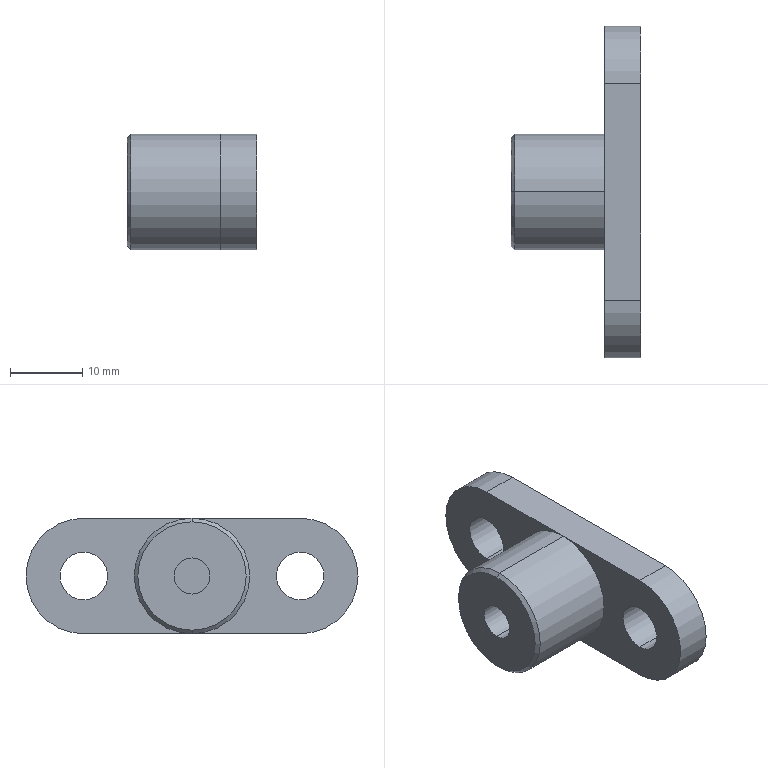Part | STEP file | HJDX-008 | 1 solid | 19 faces | box 18 x 46 x 16 mm | volume 5416 mm3 | cylinder 10 | plane 7 | cone 2 | commonest cylinder face diameters 6.6 x4 16 x4 5 x2
STEP:
#1=CARTESIAN_POINT('',(18.,-15.,-3.3));
#2=VERTEX_POINT('',#1);
#3=CARTESIAN_POINT('',(18.,-15.,3.3));
#4=VERTEX_POINT('',#3);
#5=CARTESIAN_POINT('',(18.,-15.,0.));
#6=DIRECTION('',(-1.,0.,0.));
#7=DIRECTION('',(0.,0.,1.));
#8=AXIS2_PLACEMENT_3D('',#5,#6,#7);
#9=CIRCLE('',#8,3.3);
#10=EDGE_CURVE('',#2,#4,#9,.T.);
#11=ORIENTED_EDGE('',*,*,#10,.F.);
#12=CARTESIAN_POINT('',(13.,-15.,-3.3));
#13=VERTEX_POINT('',#12);
#14=CARTESIAN_POINT('',(13.,-15.,-3.3));
#15=DIRECTION('',(-1.,0.,0.));
#16=VECTOR('',#15,1000.);
#17=LINE('',#14,#16);
#18=EDGE_CURVE('',#2,#13,#17,.T.);
#19=ORIENTED_EDGE('',*,*,#18,.T.);
#20=CARTESIAN_POINT('',(13.,-15.,3.3));
#21=VERTEX_POINT('',#20);
#22=CARTESIAN_POINT('',(13.,-15.,0.));
#23=DIRECTION('',(1.,0.,0.));
#24=DIRECTION('',(0.,0.,1.));
#25=AXIS2_PLACEMENT_3D('',#22,#23,#24);
#26=CIRCLE('',#25,3.3);
#27=EDGE_CURVE('',#21,#13,#26,.T.);
#28=ORIENTED_EDGE('',*,*,#27,.F.);
#29=CARTESIAN_POINT('',(13.,-15.,3.3));
#30=DIRECTION('',(-1.,0.,0.));
#31=VECTOR('',#30,1000.);
#32=LINE('',#29,#31);
#33=EDGE_CURVE('',#4,#21,#32,.T.);
#34=ORIENTED_EDGE('',*,*,#33,.F.);
#35=EDGE_LOOP('',(#11,#19,#28,#34));
#36=FACE_OUTER_BOUND('',#35,.T.);
#37=CARTESIAN_POINT('',(13.,-15.,0.));
#38=DIRECTION('',(-1.,0.,0.));
#39=DIRECTION('',(0.,0.,1.));
#40=AXIS2_PLACEMENT_3D('',#37,#38,#39);
#41=CYLINDRICAL_SURFACE('',#40,3.3);
#42=ADVANCED_FACE('',(#36),#41,.F.);
#43=CARTESIAN_POINT('',(18.,15.,-3.3));
#44=VERTEX_POINT('',#43);
#45=CARTESIAN_POINT('',(18.,15.,3.3));
#46=VERTEX_POINT('',#45);
#47=CARTESIAN_POINT('',(18.,15.,0.));
#48=DIRECTION('',(-1.,0.,0.));
#49=DIRECTION('',(0.,0.,1.));
#50=AXIS2_PLACEMENT_3D('',#47,#48,#49);
#51=CIRCLE('',#50,3.3);
#52=EDGE_CURVE('',#44,#46,#51,.T.);
#53=ORIENTED_EDGE('',*,*,#52,.F.);
#54=CARTESIAN_POINT('',(13.,15.,-3.3));
#55=VERTEX_POINT('',#54);
#56=CARTESIAN_POINT('',(13.,15.,-3.3));
#57=DIRECTION('',(-1.,0.,0.));
#58=VECTOR('',#57,1000.);
#59=LINE('',#56,#58);
#60=EDGE_CURVE('',#44,#55,#59,.T.);
#61=ORIENTED_EDGE('',*,*,#60,.T.);
#62=CARTESIAN_POINT('',(13.,15.,3.3));
#63=VERTEX_POINT('',#62);
#64=CARTESIAN_POINT('',(13.,15.,0.));
#65=DIRECTION('',(1.,0.,0.));
#66=DIRECTION('',(0.,0.,1.));
#67=AXIS2_PLACEMENT_3D('',#64,#65,#66);
#68=CIRCLE('',#67,3.3);
#69=EDGE_CURVE('',#63,#55,#68,.T.);
#70=ORIENTED_EDGE('',*,*,#69,.F.);
#71=CARTESIAN_POINT('',(13.,15.,3.3));
#72=DIRECTION('',(-1.,0.,0.));
#73=VECTOR('',#72,1000.);
#74=LINE('',#71,#73);
#75=EDGE_CURVE('',#46,#63,#74,.T.);
#76=ORIENTED_EDGE('',*,*,#75,.F.);
#77=EDGE_LOOP('',(#53,#61,#70,#76));
#78=FACE_OUTER_BOUND('',#77,.T.);
#79=CARTESIAN_POINT('',(13.,15.,0.));
#80=DIRECTION('',(-1.,0.,0.));
#81=DIRECTION('',(0.,0.,1.));
#82=AXIS2_PLACEMENT_3D('',#79,#80,#81);
#83=CYLINDRICAL_SURFACE('',#82,3.3);
#84=ADVANCED_FACE('',(#78),#83,.F.);
#85=CARTESIAN_POINT('',(13.,0.,8.));
#86=VERTEX_POINT('',#85);
#87=CARTESIAN_POINT('',(13.,0.,-8.));
#88=VERTEX_POINT('',#87);
#89=CARTESIAN_POINT('',(13.,0.,0.));
#90=DIRECTION('',(-1.,0.,0.));
#91=DIRECTION('',(0.,0.,1.));
#92=AXIS2_PLACEMENT_3D('',#89,#90,#91);
#93=CIRCLE('',#92,8.);
#94=EDGE_CURVE('',#86,#88,#93,.T.);
#95=ORIENTED_EDGE('',*,*,#94,.T.);
#96=CARTESIAN_POINT('',(0.5,0.,-8.));
#97=VERTEX_POINT('',#96);
#98=CARTESIAN_POINT('',(18.,0.,-8.));
#99=DIRECTION('',(-1.,0.,0.));
#100=VECTOR('',#99,1000.);
#101=LINE('',#98,#100);
#102=EDGE_CURVE('',#88,#97,#101,.T.);
#103=ORIENTED_EDGE('',*,*,#102,.T.);
#104=CARTESIAN_POINT('',(0.5,0.,8.));
#105=VERTEX_POINT('',#104);
#106=CARTESIAN_POINT('',(0.5,0.,0.));
#107=DIRECTION('',(1.,0.,0.));
#108=DIRECTION('',(0.,0.,1.));
#109=AXIS2_PLACEMENT_3D('',#106,#107,#108);
#110=CIRCLE('',#109,8.);
#111=EDGE_CURVE('',#97,#105,#110,.T.);
#112=ORIENTED_EDGE('',*,*,#111,.T.);
#113=CARTESIAN_POINT('',(18.,0.,8.));
#114=DIRECTION('',(-1.,0.,0.));
#115=VECTOR('',#114,1000.);
#116=LINE('',#113,#115);
#117=EDGE_CURVE('',#86,#105,#116,.T.);
#118=ORIENTED_EDGE('',*,*,#117,.F.);
#119=EDGE_LOOP('',(#95,#103,#112,#118));
#120=FACE_OUTER_BOUND('',#119,.T.);
#121=CARTESIAN_POINT('',(18.,0.,0.));
#122=DIRECTION('',(-1.,0.,0.));
#123=DIRECTION('',(0.,0.,1.));
#124=AXIS2_PLACEMENT_3D('',#121,#122,#123);
#125=CYLINDRICAL_SURFACE('',#124,8.);
#126=ADVANCED_FACE('',(#120),#125,.T.);
#127=CARTESIAN_POINT('',(0.,0.,-7.5));
#128=VERTEX_POINT('',#127);
#129=CARTESIAN_POINT('',(0.,0.,7.5));
#130=VERTEX_POINT('',#129);
#131=CARTESIAN_POINT('',(0.,0.,0.));
#132=DIRECTION('',(1.,0.,0.));
#133=DIRECTION('',(0.,0.,-1.));
#134=AXIS2_PLACEMENT_3D('',#131,#132,#133);
#135=CIRCLE('',#134,7.5);
#136=EDGE_CURVE('',#128,#130,#135,.T.);
#137=ORIENTED_EDGE('',*,*,#136,.T.);
#138=CARTESIAN_POINT('',(0.5,0.,8.));
#139=DIRECTION('',(0.7071,0.,0.7071));
#140=VECTOR('',#139,1000.);
#141=LINE('',#138,#140);
#142=EDGE_CURVE('',#130,#105,#141,.T.);
#143=ORIENTED_EDGE('',*,*,#142,.T.);
#144=ORIENTED_EDGE('',*,*,#111,.F.);
#145=CARTESIAN_POINT('',(0.5,0.,-8.));
#146=DIRECTION('',(0.7071,0.,-0.7071));
#147=VECTOR('',#146,1000.);
#148=LINE('',#145,#147);
#149=EDGE_CURVE('',#128,#97,#148,.T.);
#150=ORIENTED_EDGE('',*,*,#149,.F.);
#151=EDGE_LOOP('',(#137,#143,#144,#150));
#152=FACE_OUTER_BOUND('',#151,.T.);
#153=CARTESIAN_POINT('',(0.5,0.,0.));
#154=DIRECTION('',(1.,0.,0.));
#155=DIRECTION('',(0.,0.,-1.));
#156=AXIS2_PLACEMENT_3D('',#153,#154,#155);
#157=CONICAL_SURFACE('',#156,8.,0.7854);
#158=ADVANCED_FACE('',(#152),#157,.T.);
#159=CARTESIAN_POINT('',(13.,0.,-2.5));
#160=VERTEX_POINT('',#159);
#161=CARTESIAN_POINT('',(13.,0.,2.5));
#162=VERTEX_POINT('',#161);
#163=CARTESIAN_POINT('',(13.,0.,0.));
#164=DIRECTION('',(-1.,0.,0.));
#165=DIRECTION('',(0.,0.,1.));
#166=AXIS2_PLACEMENT_3D('',#163,#164,#165);
#167=CIRCLE('',#166,2.5);
#168=EDGE_CURVE('',#160,#162,#167,.T.);
#169=ORIENTED_EDGE('',*,*,#168,.F.);
#170=CARTESIAN_POINT('',(0.,0.,-2.5));
#171=VERTEX_POINT('',#170);
#172=CARTESIAN_POINT('',(0.,0.,-2.5));
#173=DIRECTION('',(-1.,0.,0.));
#174=VECTOR('',#173,1000.);
#175=LINE('',#172,#174);
#176=EDGE_CURVE('',#160,#171,#175,.T.);
#177=ORIENTED_EDGE('',*,*,#176,.T.);
#178=CARTESIAN_POINT('',(0.,0.,2.5));
#179=VERTEX_POINT('',#178);
#180=CARTESIAN_POINT('',(0.,0.,0.));
#181=DIRECTION('',(-1.,0.,0.));
#182=DIRECTION('',(0.,0.,1.));
#183=AXIS2_PLACEMENT_3D('',#180,#181,#182);
#184=CIRCLE('',#183,2.5);
#185=EDGE_CURVE('',#171,#179,#184,.T.);
#186=ORIENTED_EDGE('',*,*,#185,.T.);
#187=CARTESIAN_POINT('',(0.,0.,2.5));
#188=DIRECTION('',(-1.,0.,0.));
#189=VECTOR('',#188,1000.);
#190=LINE('',#187,#189);
#191=EDGE_CURVE('',#162,#179,#190,.T.);
#192=ORIENTED_EDGE('',*,*,#191,.F.);
#193=EDGE_LOOP('',(#169,#177,#186,#192));
#194=FACE_OUTER_BOUND('',#193,.T.);
#195=CARTESIAN_POINT('',(0.,0.,0.));
#196=DIRECTION('',(-1.,0.,0.));
#197=DIRECTION('',(0.,0.,1.));
#198=AXIS2_PLACEMENT_3D('',#195,#196,#197);
#199=CYLINDRICAL_SURFACE('',#198,2.5);
#200=ADVANCED_FACE('',(#194),#199,.F.);
#201=CARTESIAN_POINT('',(18.,-15.,0.));
#202=DIRECTION('',(-1.,0.,0.));
#203=DIRECTION('',(0.,0.,1.));
#204=AXIS2_PLACEMENT_3D('',#201,#202,#203);
#205=CIRCLE('',#204,3.3);
#206=EDGE_CURVE('',#4,#2,#205,.T.);
#207=ORIENTED_EDGE('',*,*,#206,.T.);
#208=ORIENTED_EDGE('',*,*,#10,.T.);
#209=EDGE_LOOP('',(#207,#208));
#210=FACE_BOUND('',#209,.T.);
#211=CARTESIAN_POINT('',(18.,15.,-8.));
#212=VERTEX_POINT('',#211);
#213=CARTESIAN_POINT('',(18.,15.,8.));
#214=VERTEX_POINT('',#213);
#215=CARTESIAN_POINT('',(18.,15.,0.));
#216=DIRECTION('',(1.,0.,0.));
#217=DIRECTION('',(0.,0.,-1.));
#218=AXIS2_PLACEMENT_3D('',#215,#216,#217);
#219=CIRCLE('',#218,8.);
#220=EDGE_CURVE('',#212,#214,#219,.T.);
#221=ORIENTED_EDGE('',*,*,#220,.T.);
#222=CARTESIAN_POINT('',(18.,-15.,8.));
#223=VERTEX_POINT('',#222);
#224=CARTESIAN_POINT('',(18.,0.,8.));
#225=DIRECTION('',(0.,-1.,0.));
#226=VECTOR('',#225,1000.);
#227=LINE('',#224,#226);
#228=EDGE_CURVE('',#214,#223,#227,.T.);
#229=ORIENTED_EDGE('',*,*,#228,.T.);
#230=CARTESIAN_POINT('',(18.,-15.,-8.));
#231=VERTEX_POINT('',#230);
#232=CARTESIAN_POINT('',(18.,-15.,0.));
#233=DIRECTION('',(1.,0.,0.));
#234=DIRECTION('',(0.,0.,-1.));
#235=AXIS2_PLACEMENT_3D('',#232,#233,#234);
#236=CIRCLE('',#235,8.);
#237=EDGE_CURVE('',#223,#231,#236,.T.);
#238=ORIENTED_EDGE('',*,*,#237,.T.);
#239=CARTESIAN_POINT('',(18.,0.,-8.));
#240=DIRECTION('',(0.,1.,0.));
#241=VECTOR('',#240,1000.);
#242=LINE('',#239,#241);
#243=EDGE_CURVE('',#231,#212,#242,.T.);
#244=ORIENTED_EDGE('',*,*,#243,.T.);
#245=EDGE_LOOP('',(#221,#229,#238,#244));
#246=FACE_OUTER_BOUND('',#245,.T.);
#247=CARTESIAN_POINT('',(18.,15.,0.));
#248=DIRECTION('',(-1.,0.,0.));
#249=DIRECTION('',(0.,0.,1.));
#250=AXIS2_PLACEMENT_3D('',#247,#248,#249);
#251=CIRCLE('',#250,3.3);
#252=EDGE_CURVE('',#46,#44,#251,.T.);
#253=ORIENTED_EDGE('',*,*,#252,.T.);
#254=ORIENTED_EDGE('',*,*,#52,.T.);
#255=EDGE_LOOP('',(#253,#254));
#256=FACE_BOUND('',#255,.T.);
#257=CARTESIAN_POINT('',(18.,0.,0.));
#258=DIRECTION('',(1.,0.,0.));
#259=DIRECTION('',(0.,0.,-1.));
#260=AXIS2_PLACEMENT_3D('',#257,#258,#259);
#261=PLANE('',#260);
#262=ADVANCED_FACE('',(#210,#246,#256),#261,.T.);
#263=ORIENTED_EDGE('',*,*,#18,.F.);
#264=ORIENTED_EDGE('',*,*,#206,.F.);
#265=ORIENTED_EDGE('',*,*,#33,.T.);
#266=CARTESIAN_POINT('',(13.,-15.,0.));
#267=DIRECTION('',(1.,0.,0.));
#268=DIRECTION('',(0.,0.,1.));
#269=AXIS2_PLACEMENT_3D('',#266,#267,#268);
#270=CIRCLE('',#269,3.3);
#271=EDGE_CURVE('',#13,#21,#270,.T.);
#272=ORIENTED_EDGE('',*,*,#271,.F.);
#273=EDGE_LOOP('',(#263,#264,#265,#272));
#274=FACE_OUTER_BOUND('',#273,.T.);
#275=CARTESIAN_POINT('',(13.,-15.,0.));
#276=DIRECTION('',(-1.,0.,0.));
#277=DIRECTION('',(0.,0.,1.));
#278=AXIS2_PLACEMENT_3D('',#275,#276,#277);
#279=CYLINDRICAL_SURFACE('',#278,3.3);
#280=ADVANCED_FACE('',(#274),#279,.F.);
#281=ORIENTED_EDGE('',*,*,#228,.F.);
#282=CARTESIAN_POINT('',(13.,15.,8.));
#283=VERTEX_POINT('',#282);
#284=CARTESIAN_POINT('',(13.,15.,8.));
#285=DIRECTION('',(-1.,0.,0.));
#286=VECTOR('',#285,1000.);
#287=LINE('',#284,#286);
#288=EDGE_CURVE('',#214,#283,#287,.T.);
#289=ORIENTED_EDGE('',*,*,#288,.T.);
#290=CARTESIAN_POINT('',(13.,-15.,8.));
#291=DIRECTION('',(0.,-1.,0.));
#292=VECTOR('',#291,1000.);
#293=LINE('',#290,#292);
#294=EDGE_CURVE('',#283,#86,#293,.T.);
#295=ORIENTED_EDGE('',*,*,#294,.T.);
#296=CARTESIAN_POINT('',(13.,-15.,8.));
#297=VERTEX_POINT('',#296);
#298=CARTESIAN_POINT('',(13.,-15.,8.));
#299=DIRECTION('',(0.,-1.,0.));
#300=VECTOR('',#299,1000.);
#301=LINE('',#298,#300);
#302=EDGE_CURVE('',#86,#297,#301,.T.);
#303=ORIENTED_EDGE('',*,*,#302,.T.);
#304=CARTESIAN_POINT('',(13.,-15.,8.));
#305=DIRECTION('',(1.,0.,0.));
#306=VECTOR('',#305,1000.);
#307=LINE('',#304,#306);
#308=EDGE_CURVE('',#297,#223,#307,.T.);
#309=ORIENTED_EDGE('',*,*,#308,.T.);
#310=EDGE_LOOP('',(#281,#289,#295,#303,#309));
#311=FACE_OUTER_BOUND('',#310,.T.);
#312=CARTESIAN_POINT('',(13.,-15.,8.));
#313=DIRECTION('',(0.,0.,1.));
#314=DIRECTION('',(0.,-1.,0.));
#315=AXIS2_PLACEMENT_3D('',#312,#313,#314);
#316=PLANE('',#315);
#317=ADVANCED_FACE('',(#311),#316,.T.);
#318=CARTESIAN_POINT('',(13.,15.,-8.));
#319=VERTEX_POINT('',#318);
#320=CARTESIAN_POINT('',(13.,15.,0.));
#321=DIRECTION('',(1.,0.,0.));
#322=DIRECTION('',(0.,0.,-1.));
#323=AXIS2_PLACEMENT_3D('',#320,#321,#322);
#324=CIRCLE('',#323,8.);
#325=EDGE_CURVE('',#319,#283,#324,.T.);
#326=ORIENTED_EDGE('',*,*,#325,.T.);
#327=ORIENTED_EDGE('',*,*,#288,.F.);
#328=ORIENTED_EDGE('',*,*,#220,.F.);
#329=CARTESIAN_POINT('',(13.,15.,-8.));
#330=DIRECTION('',(-1.,0.,0.));
#331=VECTOR('',#330,1000.);
#332=LINE('',#329,#331);
#333=EDGE_CURVE('',#212,#319,#332,.T.);
#334=ORIENTED_EDGE('',*,*,#333,.T.);
#335=EDGE_LOOP('',(#326,#327,#328,#334));
#336=FACE_OUTER_BOUND('',#335,.T.);
#337=CARTESIAN_POINT('',(13.,15.,0.));
#338=DIRECTION('',(1.,0.,0.));
#339=DIRECTION('',(0.,0.,-1.));
#340=AXIS2_PLACEMENT_3D('',#337,#338,#339);
#341=CYLINDRICAL_SURFACE('',#340,8.);
#342=ADVANCED_FACE('',(#336),#341,.T.);
#343=ORIENTED_EDGE('',*,*,#243,.F.);
#344=CARTESIAN_POINT('',(13.,-15.,-8.));
#345=VERTEX_POINT('',#344);
#346=CARTESIAN_POINT('',(13.,-15.,-8.));
#347=DIRECTION('',(-1.,0.,0.));
#348=VECTOR('',#347,1000.);
#349=LINE('',#346,#348);
#350=EDGE_CURVE('',#231,#345,#349,.T.);
#351=ORIENTED_EDGE('',*,*,#350,.T.);
#352=CARTESIAN_POINT('',(13.,-15.,-8.));
#353=DIRECTION('',(0.,1.,0.));
#354=VECTOR('',#353,1000.);
#355=LINE('',#352,#354);
#356=EDGE_CURVE('',#345,#88,#355,.T.);
#357=ORIENTED_EDGE('',*,*,#356,.T.);
#358=CARTESIAN_POINT('',(13.,-15.,-8.));
#359=DIRECTION('',(0.,1.,0.));
#360=VECTOR('',#359,1000.);
#361=LINE('',#358,#360);
#362=EDGE_CURVE('',#88,#319,#361,.T.);
#363=ORIENTED_EDGE('',*,*,#362,.T.);
#364=ORIENTED_EDGE('',*,*,#333,.F.);
#365=EDGE_LOOP('',(#343,#351,#357,#363,#364));
#366=FACE_OUTER_BOUND('',#365,.T.);
#367=CARTESIAN_POINT('',(13.,-15.,-8.));
#368=DIRECTION('',(0.,0.,-1.));
#369=DIRECTION('',(0.,1.,0.));
#370=AXIS2_PLACEMENT_3D('',#367,#368,#369);
#371=PLANE('',#370);
#372=ADVANCED_FACE('',(#366),#371,.T.);
#373=CARTESIAN_POINT('',(13.,-15.,0.));
#374=DIRECTION('',(1.,0.,0.));
#375=DIRECTION('',(0.,0.,-1.));
#376=AXIS2_PLACEMENT_3D('',#373,#374,#375);
#377=CIRCLE('',#376,8.);
#378=EDGE_CURVE('',#297,#345,#377,.T.);
#379=ORIENTED_EDGE('',*,*,#378,.T.);
#380=ORIENTED_EDGE('',*,*,#350,.F.);
#381=ORIENTED_EDGE('',*,*,#237,.F.);
#382=ORIENTED_EDGE('',*,*,#308,.F.);
#383=EDGE_LOOP('',(#379,#380,#381,#382));
#384=FACE_OUTER_BOUND('',#383,.T.);
#385=CARTESIAN_POINT('',(13.,-15.,0.));
#386=DIRECTION('',(1.,0.,0.));
#387=DIRECTION('',(0.,0.,-1.));
#388=AXIS2_PLACEMENT_3D('',#385,#386,#387);
#389=CYLINDRICAL_SURFACE('',#388,8.);
#390=ADVANCED_FACE('',(#384),#389,.T.);
#391=ORIENTED_EDGE('',*,*,#60,.F.);
#392=ORIENTED_EDGE('',*,*,#252,.F.);
#393=ORIENTED_EDGE('',*,*,#75,.T.);
#394=CARTESIAN_POINT('',(13.,15.,0.));
#395=DIRECTION('',(1.,0.,0.));
#396=DIRECTION('',(0.,0.,1.));
#397=AXIS2_PLACEMENT_3D('',#394,#395,#396);
#398=CIRCLE('',#397,3.3);
#399=EDGE_CURVE('',#55,#63,#398,.T.);
#400=ORIENTED_EDGE('',*,*,#399,.F.);
#401=EDGE_LOOP('',(#391,#392,#393,#400));
#402=FACE_OUTER_BOUND('',#401,.T.);
#403=CARTESIAN_POINT('',(13.,15.,0.));
#404=DIRECTION('',(-1.,0.,0.));
#405=DIRECTION('',(0.,0.,1.));
#406=AXIS2_PLACEMENT_3D('',#403,#404,#405);
#407=CYLINDRICAL_SURFACE('',#406,3.3);
#408=ADVANCED_FACE('',(#402),#407,.F.);
#409=CARTESIAN_POINT('',(13.,0.,0.));
#410=DIRECTION('',(-1.,0.,0.));
#411=DIRECTION('',(0.,0.,1.));
#412=AXIS2_PLACEMENT_3D('',#409,#410,#411);
#413=CIRCLE('',#412,8.);
#414=EDGE_CURVE('',#88,#86,#413,.T.);
#415=ORIENTED_EDGE('',*,*,#414,.F.);
#416=ORIENTED_EDGE('',*,*,#356,.F.);
#417=ORIENTED_EDGE('',*,*,#378,.F.);
#418=ORIENTED_EDGE('',*,*,#302,.F.);
#419=EDGE_LOOP('',(#415,#416,#417,#418));
#420=FACE_OUTER_BOUND('',#419,.T.);
#421=ORIENTED_EDGE('',*,*,#27,.T.);
#422=ORIENTED_EDGE('',*,*,#271,.T.);
#423=EDGE_LOOP('',(#421,#422));
#424=FACE_BOUND('',#423,.T.);
#425=CARTESIAN_POINT('',(13.,-15.,0.));
#426=DIRECTION('',(1.,0.,0.));
#427=DIRECTION('',(0.,0.,-1.));
#428=AXIS2_PLACEMENT_3D('',#425,#426,#427);
#429=PLANE('',#428);
#430=ADVANCED_FACE('',(#420,#424),#429,.F.);
#431=ORIENTED_EDGE('',*,*,#94,.F.);
#432=ORIENTED_EDGE('',*,*,#294,.F.);
#433=ORIENTED_EDGE('',*,*,#325,.F.);
#434=ORIENTED_EDGE('',*,*,#362,.F.);
#435=EDGE_LOOP('',(#431,#432,#433,#434));
#436=FACE_OUTER_BOUND('',#435,.T.);
#437=ORIENTED_EDGE('',*,*,#69,.T.);
#438=ORIENTED_EDGE('',*,*,#399,.T.);
#439=EDGE_LOOP('',(#437,#438));
#440=FACE_BOUND('',#439,.T.);
#441=CARTESIAN_POINT('',(13.,-15.,0.));
#442=DIRECTION('',(1.,0.,0.));
#443=DIRECTION('',(0.,0.,-1.));
#444=AXIS2_PLACEMENT_3D('',#441,#442,#443);
#445=PLANE('',#444);
#446=ADVANCED_FACE('',(#436,#440),#445,.F.);
#447=ORIENTED_EDGE('',*,*,#102,.F.);
#448=ORIENTED_EDGE('',*,*,#414,.T.);
#449=ORIENTED_EDGE('',*,*,#117,.T.);
#450=CARTESIAN_POINT('',(0.5,0.,0.));
#451=DIRECTION('',(1.,0.,0.));
#452=DIRECTION('',(0.,0.,1.));
#453=AXIS2_PLACEMENT_3D('',#450,#451,#452);
#454=CIRCLE('',#453,8.);
#455=EDGE_CURVE('',#105,#97,#454,.T.);
#456=ORIENTED_EDGE('',*,*,#455,.T.);
#457=EDGE_LOOP('',(#447,#448,#449,#456));
#458=FACE_OUTER_BOUND('',#457,.T.);
#459=CARTESIAN_POINT('',(18.,0.,0.));
#460=DIRECTION('',(-1.,0.,0.));
#461=DIRECTION('',(0.,0.,1.));
#462=AXIS2_PLACEMENT_3D('',#459,#460,#461);
#463=CYLINDRICAL_SURFACE('',#462,8.);
#464=ADVANCED_FACE('',(#458),#463,.T.);
#465=ORIENTED_EDGE('',*,*,#142,.F.);
#466=CARTESIAN_POINT('',(0.,0.,0.));
#467=DIRECTION('',(1.,0.,0.));
#468=DIRECTION('',(0.,0.,-1.));
#469=AXIS2_PLACEMENT_3D('',#466,#467,#468);
#470=CIRCLE('',#469,7.5);
#471=EDGE_CURVE('',#130,#128,#470,.T.);
#472=ORIENTED_EDGE('',*,*,#471,.T.);
#473=ORIENTED_EDGE('',*,*,#149,.T.);
#474=ORIENTED_EDGE('',*,*,#455,.F.);
#475=EDGE_LOOP('',(#465,#472,#473,#474));
#476=FACE_OUTER_BOUND('',#475,.T.);
#477=CARTESIAN_POINT('',(0.5,0.,0.));
#478=DIRECTION('',(1.,0.,0.));
#479=DIRECTION('',(0.,0.,-1.));
#480=AXIS2_PLACEMENT_3D('',#477,#478,#479);
#481=CONICAL_SURFACE('',#480,8.,0.7854);
#482=ADVANCED_FACE('',(#476),#481,.T.);
#483=ORIENTED_EDGE('',*,*,#136,.F.);
#484=ORIENTED_EDGE('',*,*,#471,.F.);
#485=EDGE_LOOP('',(#483,#484));
#486=FACE_OUTER_BOUND('',#485,.T.);
#487=CARTESIAN_POINT('',(0.,0.,0.));
#488=DIRECTION('',(-1.,0.,0.));
#489=DIRECTION('',(0.,0.,1.));
#490=AXIS2_PLACEMENT_3D('',#487,#488,#489);
#491=CIRCLE('',#490,2.5);
#492=EDGE_CURVE('',#179,#171,#491,.T.);
#493=ORIENTED_EDGE('',*,*,#492,.F.);
#494=ORIENTED_EDGE('',*,*,#185,.F.);
#495=EDGE_LOOP('',(#493,#494));
#496=FACE_BOUND('',#495,.T.);
#497=CARTESIAN_POINT('',(0.,0.,0.));
#498=DIRECTION('',(1.,0.,0.));
#499=DIRECTION('',(0.,0.,-1.));
#500=AXIS2_PLACEMENT_3D('',#497,#498,#499);
#501=PLANE('',#500);
#502=ADVANCED_FACE('',(#486,#496),#501,.F.);
#503=ORIENTED_EDGE('',*,*,#176,.F.);
#504=CARTESIAN_POINT('',(13.,0.,0.));
#505=DIRECTION('',(-1.,0.,0.));
#506=DIRECTION('',(0.,0.,1.));
#507=AXIS2_PLACEMENT_3D('',#504,#505,#506);
#508=CIRCLE('',#507,2.5);
#509=EDGE_CURVE('',#162,#160,#508,.T.);
#510=ORIENTED_EDGE('',*,*,#509,.F.);
#511=ORIENTED_EDGE('',*,*,#191,.T.);
#512=ORIENTED_EDGE('',*,*,#492,.T.);
#513=EDGE_LOOP('',(#503,#510,#511,#512));
#514=FACE_OUTER_BOUND('',#513,.T.);
#515=CARTESIAN_POINT('',(0.,0.,0.));
#516=DIRECTION('',(-1.,0.,0.));
#517=DIRECTION('',(0.,0.,1.));
#518=AXIS2_PLACEMENT_3D('',#515,#516,#517);
#519=CYLINDRICAL_SURFACE('',#518,2.5);
#520=ADVANCED_FACE('',(#514),#519,.F.);
#521=ORIENTED_EDGE('',*,*,#509,.T.);
#522=ORIENTED_EDGE('',*,*,#168,.T.);
#523=EDGE_LOOP('',(#521,#522));
#524=FACE_OUTER_BOUND('',#523,.T.);
#525=CARTESIAN_POINT('',(13.,-15.,0.));
#526=DIRECTION('',(1.,0.,0.));
#527=DIRECTION('',(0.,0.,-1.));
#528=AXIS2_PLACEMENT_3D('',#525,#526,#527);
#529=PLANE('',#528);
#530=ADVANCED_FACE('',(#524),#529,.F.);
#531=CLOSED_SHELL('',(#42,#84,#126,#158,#200,#262,#280,#317,#342,#372,#390,#408,#430,#446,#464,#482,#502,#520,#530));
#532=MANIFOLD_SOLID_BREP('',#531);
#533=CARTESIAN_POINT('',(0.,0.,0.));
#534=DIRECTION('',(0.,0.,1.));
#535=DIRECTION('',(1.,0.,0.));
#536=AXIS2_PLACEMENT_3D('',#533,#534,#535);
#537=(LENGTH_UNIT()NAMED_UNIT(*)SI_UNIT(.MILLI.,.METRE.));
#538=UNCERTAINTY_MEASURE_WITH_UNIT(LENGTH_MEASURE(0.00001),#537,'','');
#539=(NAMED_UNIT(*)PLANE_ANGLE_UNIT()SI_UNIT($,.RADIAN.));
#540=(NAMED_UNIT(*)SI_UNIT($,.STERADIAN.)SOLID_ANGLE_UNIT());
#541=(GEOMETRIC_REPRESENTATION_CONTEXT(3)GLOBAL_UNCERTAINTY_ASSIGNED_CONTEXT((#538))GLOBAL_UNIT_ASSIGNED_CONTEXT((#537,#539,#540))REPRESENTATION_CONTEXT('',''));
#542=ADVANCED_BREP_SHAPE_REPRESENTATION('',(#532,#536),#541);